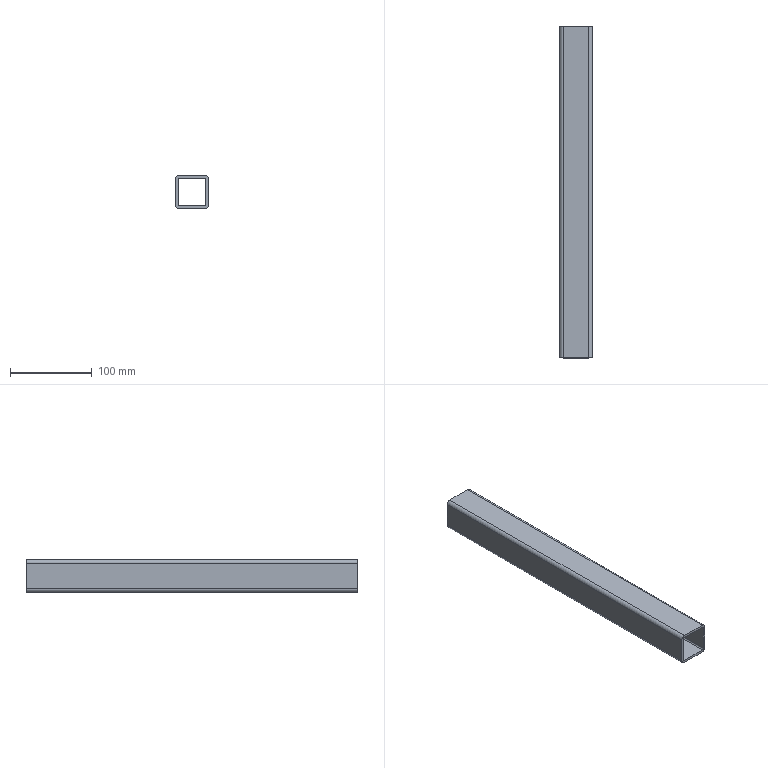Part | 1 solid | 18 faces | box 40 x 405 x 40 mm | volume 173562 mm3 | plane 10 | cylinder 8 | commonest cylinder face diameters 3 x4 9 x4
STEP:
#1=CARTESIAN_POINT('',(20.,0.,15.5));
#2=VERTEX_POINT('',#1);
#3=CARTESIAN_POINT('',(20.,0.,-15.5));
#4=VERTEX_POINT('',#3);
#5=CARTESIAN_POINT('',(20.,0.,20.));
#6=DIRECTION('',(0.,0.,-1.));
#7=VECTOR('',#6,1000.);
#8=LINE('',#5,#7);
#9=EDGE_CURVE('',#2,#4,#8,.T.);
#10=ORIENTED_EDGE('',*,*,#9,.T.);
#11=CARTESIAN_POINT('',(20.,405.,-15.5));
#12=VERTEX_POINT('',#11);
#13=CARTESIAN_POINT('',(20.,405.,-15.5));
#14=DIRECTION('',(0.,1.,0.));
#15=VECTOR('',#14,1000.);
#16=LINE('',#13,#15);
#17=EDGE_CURVE('',#4,#12,#16,.T.);
#18=ORIENTED_EDGE('',*,*,#17,.T.);
#19=CARTESIAN_POINT('',(20.,405.,15.5));
#20=VERTEX_POINT('',#19);
#21=CARTESIAN_POINT('',(20.,405.,20.));
#22=DIRECTION('',(0.,0.,-1.));
#23=VECTOR('',#22,1000.);
#24=LINE('',#21,#23);
#25=EDGE_CURVE('',#20,#12,#24,.T.);
#26=ORIENTED_EDGE('',*,*,#25,.F.);
#27=CARTESIAN_POINT('',(20.,405.,15.5));
#28=DIRECTION('',(0.,-1.,0.));
#29=VECTOR('',#28,1000.);
#30=LINE('',#27,#29);
#31=EDGE_CURVE('',#20,#2,#30,.T.);
#32=ORIENTED_EDGE('',*,*,#31,.T.);
#33=EDGE_LOOP('',(#10,#18,#26,#32));
#34=FACE_OUTER_BOUND('',#33,.T.);
#35=CARTESIAN_POINT('',(20.,405.,20.));
#36=DIRECTION('',(-1.,0.,0.));
#37=DIRECTION('',(0.,0.,1.));
#38=AXIS2_PLACEMENT_3D('',#35,#36,#37);
#39=PLANE('',#38);
#40=ADVANCED_FACE('',(#34),#39,.F.);
#41=CARTESIAN_POINT('',(15.5,0.,-20.));
#42=VERTEX_POINT('',#41);
#43=CARTESIAN_POINT('',(-15.5,0.,-20.));
#44=VERTEX_POINT('',#43);
#45=CARTESIAN_POINT('',(-20.,0.,-20.));
#46=DIRECTION('',(-1.,0.,0.));
#47=VECTOR('',#46,1000.);
#48=LINE('',#45,#47);
#49=EDGE_CURVE('',#42,#44,#48,.T.);
#50=ORIENTED_EDGE('',*,*,#49,.T.);
#51=CARTESIAN_POINT('',(-15.5,405.,-20.));
#52=VERTEX_POINT('',#51);
#53=CARTESIAN_POINT('',(-15.5,405.,-20.));
#54=DIRECTION('',(0.,1.,0.));
#55=VECTOR('',#54,1000.);
#56=LINE('',#53,#55);
#57=EDGE_CURVE('',#44,#52,#56,.T.);
#58=ORIENTED_EDGE('',*,*,#57,.T.);
#59=CARTESIAN_POINT('',(15.5,405.,-20.));
#60=VERTEX_POINT('',#59);
#61=CARTESIAN_POINT('',(-20.,405.,-20.));
#62=DIRECTION('',(-1.,0.,0.));
#63=VECTOR('',#62,1000.);
#64=LINE('',#61,#63);
#65=EDGE_CURVE('',#60,#52,#64,.T.);
#66=ORIENTED_EDGE('',*,*,#65,.F.);
#67=CARTESIAN_POINT('',(15.5,405.,-20.));
#68=DIRECTION('',(0.,-1.,0.));
#69=VECTOR('',#68,1000.);
#70=LINE('',#67,#69);
#71=EDGE_CURVE('',#60,#42,#70,.T.);
#72=ORIENTED_EDGE('',*,*,#71,.T.);
#73=EDGE_LOOP('',(#50,#58,#66,#72));
#74=FACE_OUTER_BOUND('',#73,.T.);
#75=CARTESIAN_POINT('',(-20.,405.,-20.));
#76=DIRECTION('',(0.,0.,1.));
#77=DIRECTION('',(1.,0.,0.));
#78=AXIS2_PLACEMENT_3D('',#75,#76,#77);
#79=PLANE('',#78);
#80=ADVANCED_FACE('',(#74),#79,.F.);
#81=CARTESIAN_POINT('',(-20.,0.,-15.5));
#82=VERTEX_POINT('',#81);
#83=CARTESIAN_POINT('',(-20.,0.,15.5));
#84=VERTEX_POINT('',#83);
#85=CARTESIAN_POINT('',(-20.,0.,20.));
#86=DIRECTION('',(0.,0.,1.));
#87=VECTOR('',#86,1000.);
#88=LINE('',#85,#87);
#89=EDGE_CURVE('',#82,#84,#88,.T.);
#90=ORIENTED_EDGE('',*,*,#89,.T.);
#91=CARTESIAN_POINT('',(-20.,405.,15.5));
#92=VERTEX_POINT('',#91);
#93=CARTESIAN_POINT('',(-20.,405.,15.5));
#94=DIRECTION('',(0.,1.,0.));
#95=VECTOR('',#94,1000.);
#96=LINE('',#93,#95);
#97=EDGE_CURVE('',#84,#92,#96,.T.);
#98=ORIENTED_EDGE('',*,*,#97,.T.);
#99=CARTESIAN_POINT('',(-20.,405.,-15.5));
#100=VERTEX_POINT('',#99);
#101=CARTESIAN_POINT('',(-20.,405.,20.));
#102=DIRECTION('',(0.,0.,1.));
#103=VECTOR('',#102,1000.);
#104=LINE('',#101,#103);
#105=EDGE_CURVE('',#100,#92,#104,.T.);
#106=ORIENTED_EDGE('',*,*,#105,.F.);
#107=CARTESIAN_POINT('',(-20.,405.,-15.5));
#108=DIRECTION('',(0.,-1.,0.));
#109=VECTOR('',#108,1000.);
#110=LINE('',#107,#109);
#111=EDGE_CURVE('',#100,#82,#110,.T.);
#112=ORIENTED_EDGE('',*,*,#111,.T.);
#113=EDGE_LOOP('',(#90,#98,#106,#112));
#114=FACE_OUTER_BOUND('',#113,.T.);
#115=CARTESIAN_POINT('',(-20.,405.,20.));
#116=DIRECTION('',(1.,0.,0.));
#117=DIRECTION('',(0.,0.,-1.));
#118=AXIS2_PLACEMENT_3D('',#115,#116,#117);
#119=PLANE('',#118);
#120=ADVANCED_FACE('',(#114),#119,.F.);
#121=CARTESIAN_POINT('',(-15.5,405.,20.));
#122=VERTEX_POINT('',#121);
#123=CARTESIAN_POINT('',(15.5,405.,20.));
#124=VERTEX_POINT('',#123);
#125=CARTESIAN_POINT('',(-20.,405.,20.));
#126=DIRECTION('',(1.,0.,0.));
#127=VECTOR('',#126,1000.);
#128=LINE('',#125,#127);
#129=EDGE_CURVE('',#122,#124,#128,.T.);
#130=ORIENTED_EDGE('',*,*,#129,.F.);
#131=CARTESIAN_POINT('',(-15.5,0.,20.));
#132=VERTEX_POINT('',#131);
#133=CARTESIAN_POINT('',(-15.5,405.,20.));
#134=DIRECTION('',(0.,-1.,0.));
#135=VECTOR('',#134,1000.);
#136=LINE('',#133,#135);
#137=EDGE_CURVE('',#122,#132,#136,.T.);
#138=ORIENTED_EDGE('',*,*,#137,.T.);
#139=CARTESIAN_POINT('',(15.5,0.,20.));
#140=VERTEX_POINT('',#139);
#141=CARTESIAN_POINT('',(-20.,0.,20.));
#142=DIRECTION('',(1.,0.,0.));
#143=VECTOR('',#142,1000.);
#144=LINE('',#141,#143);
#145=EDGE_CURVE('',#132,#140,#144,.T.);
#146=ORIENTED_EDGE('',*,*,#145,.T.);
#147=CARTESIAN_POINT('',(15.5,405.,20.));
#148=DIRECTION('',(0.,1.,0.));
#149=VECTOR('',#148,1000.);
#150=LINE('',#147,#149);
#151=EDGE_CURVE('',#140,#124,#150,.T.);
#152=ORIENTED_EDGE('',*,*,#151,.T.);
#153=EDGE_LOOP('',(#130,#138,#146,#152));
#154=FACE_OUTER_BOUND('',#153,.T.);
#155=CARTESIAN_POINT('',(-20.,405.,20.));
#156=DIRECTION('',(0.,0.,-1.));
#157=DIRECTION('',(-1.,0.,0.));
#158=AXIS2_PLACEMENT_3D('',#155,#156,#157);
#159=PLANE('',#158);
#160=ADVANCED_FACE('',(#154),#159,.F.);
#161=CARTESIAN_POINT('',(-17.,405.,-15.5));
#162=VERTEX_POINT('',#161);
#163=CARTESIAN_POINT('',(-17.,405.,15.5));
#164=VERTEX_POINT('',#163);
#165=CARTESIAN_POINT('',(-17.,405.,-15.5));
#166=DIRECTION('',(0.,0.,1.));
#167=VECTOR('',#166,1000.);
#168=LINE('',#165,#167);
#169=EDGE_CURVE('',#162,#164,#168,.T.);
#170=ORIENTED_EDGE('',*,*,#169,.F.);
#171=CARTESIAN_POINT('',(-15.5,405.,-17.));
#172=VERTEX_POINT('',#171);
#173=CARTESIAN_POINT('',(-15.5,405.,-15.5));
#174=DIRECTION('',(0.,1.,0.));
#175=DIRECTION('',(0.,0.,1.));
#176=AXIS2_PLACEMENT_3D('',#173,#174,#175);
#177=CIRCLE('',#176,1.5);
#178=EDGE_CURVE('',#172,#162,#177,.T.);
#179=ORIENTED_EDGE('',*,*,#178,.F.);
#180=CARTESIAN_POINT('',(15.5,405.,-17.));
#181=VERTEX_POINT('',#180);
#182=CARTESIAN_POINT('',(15.5,405.,-17.));
#183=DIRECTION('',(-1.,0.,0.));
#184=VECTOR('',#183,1000.);
#185=LINE('',#182,#184);
#186=EDGE_CURVE('',#181,#172,#185,.T.);
#187=ORIENTED_EDGE('',*,*,#186,.F.);
#188=CARTESIAN_POINT('',(17.,405.,-15.5));
#189=VERTEX_POINT('',#188);
#190=CARTESIAN_POINT('',(15.5,405.,-15.5));
#191=DIRECTION('',(0.,1.,0.));
#192=DIRECTION('',(0.,0.,1.));
#193=AXIS2_PLACEMENT_3D('',#190,#191,#192);
#194=CIRCLE('',#193,1.5);
#195=EDGE_CURVE('',#189,#181,#194,.T.);
#196=ORIENTED_EDGE('',*,*,#195,.F.);
#197=CARTESIAN_POINT('',(17.,405.,15.5));
#198=VERTEX_POINT('',#197);
#199=CARTESIAN_POINT('',(17.,405.,15.5));
#200=DIRECTION('',(0.,0.,-1.));
#201=VECTOR('',#200,1000.);
#202=LINE('',#199,#201);
#203=EDGE_CURVE('',#198,#189,#202,.T.);
#204=ORIENTED_EDGE('',*,*,#203,.F.);
#205=CARTESIAN_POINT('',(15.5,405.,17.));
#206=VERTEX_POINT('',#205);
#207=CARTESIAN_POINT('',(15.5,405.,15.5));
#208=DIRECTION('',(0.,1.,0.));
#209=DIRECTION('',(0.,0.,1.));
#210=AXIS2_PLACEMENT_3D('',#207,#208,#209);
#211=CIRCLE('',#210,1.5);
#212=EDGE_CURVE('',#206,#198,#211,.T.);
#213=ORIENTED_EDGE('',*,*,#212,.F.);
#214=CARTESIAN_POINT('',(-15.5,405.,17.));
#215=VERTEX_POINT('',#214);
#216=CARTESIAN_POINT('',(-15.5,405.,17.));
#217=DIRECTION('',(1.,0.,0.));
#218=VECTOR('',#217,1000.);
#219=LINE('',#216,#218);
#220=EDGE_CURVE('',#215,#206,#219,.T.);
#221=ORIENTED_EDGE('',*,*,#220,.F.);
#222=CARTESIAN_POINT('',(-15.5,405.,15.5));
#223=DIRECTION('',(0.,1.,0.));
#224=DIRECTION('',(0.,0.,1.));
#225=AXIS2_PLACEMENT_3D('',#222,#223,#224);
#226=CIRCLE('',#225,1.5);
#227=EDGE_CURVE('',#164,#215,#226,.T.);
#228=ORIENTED_EDGE('',*,*,#227,.F.);
#229=EDGE_LOOP('',(#170,#179,#187,#196,#204,#213,#221,#228));
#230=FACE_BOUND('',#229,.T.);
#231=ORIENTED_EDGE('',*,*,#105,.T.);
#232=CARTESIAN_POINT('',(-15.5,405.,15.5));
#233=DIRECTION('',(0.,1.,0.));
#234=DIRECTION('',(0.,0.,-1.));
#235=AXIS2_PLACEMENT_3D('',#232,#233,#234);
#236=CIRCLE('',#235,4.5);
#237=EDGE_CURVE('',#92,#122,#236,.T.);
#238=ORIENTED_EDGE('',*,*,#237,.T.);
#239=ORIENTED_EDGE('',*,*,#129,.T.);
#240=CARTESIAN_POINT('',(15.5,405.,15.5));
#241=DIRECTION('',(0.,1.,0.));
#242=DIRECTION('',(0.,0.,-1.));
#243=AXIS2_PLACEMENT_3D('',#240,#241,#242);
#244=CIRCLE('',#243,4.5);
#245=EDGE_CURVE('',#124,#20,#244,.T.);
#246=ORIENTED_EDGE('',*,*,#245,.T.);
#247=ORIENTED_EDGE('',*,*,#25,.T.);
#248=CARTESIAN_POINT('',(15.5,405.,-15.5));
#249=DIRECTION('',(0.,1.,0.));
#250=DIRECTION('',(0.,0.,-1.));
#251=AXIS2_PLACEMENT_3D('',#248,#249,#250);
#252=CIRCLE('',#251,4.5);
#253=EDGE_CURVE('',#12,#60,#252,.T.);
#254=ORIENTED_EDGE('',*,*,#253,.T.);
#255=ORIENTED_EDGE('',*,*,#65,.T.);
#256=CARTESIAN_POINT('',(-15.5,405.,-15.5));
#257=DIRECTION('',(0.,1.,0.));
#258=DIRECTION('',(0.,0.,-1.));
#259=AXIS2_PLACEMENT_3D('',#256,#257,#258);
#260=CIRCLE('',#259,4.5);
#261=EDGE_CURVE('',#52,#100,#260,.T.);
#262=ORIENTED_EDGE('',*,*,#261,.T.);
#263=EDGE_LOOP('',(#231,#238,#239,#246,#247,#254,#255,#262));
#264=FACE_OUTER_BOUND('',#263,.T.);
#265=CARTESIAN_POINT('',(0.,405.,0.));
#266=DIRECTION('',(0.,-1.,0.));
#267=DIRECTION('',(0.,0.,-1.));
#268=AXIS2_PLACEMENT_3D('',#265,#266,#267);
#269=PLANE('',#268);
#270=ADVANCED_FACE('',(#230,#264),#269,.F.);
#271=CARTESIAN_POINT('',(-15.5,0.,-17.));
#272=VERTEX_POINT('',#271);
#273=CARTESIAN_POINT('',(-17.,0.,-15.5));
#274=VERTEX_POINT('',#273);
#275=CARTESIAN_POINT('',(-15.5,0.,-15.5));
#276=DIRECTION('',(0.,1.,0.));
#277=DIRECTION('',(0.,0.,1.));
#278=AXIS2_PLACEMENT_3D('',#275,#276,#277);
#279=CIRCLE('',#278,1.5);
#280=EDGE_CURVE('',#272,#274,#279,.T.);
#281=ORIENTED_EDGE('',*,*,#280,.T.);
#282=CARTESIAN_POINT('',(-17.,0.,15.5));
#283=VERTEX_POINT('',#282);
#284=CARTESIAN_POINT('',(-17.,0.,-15.5));
#285=DIRECTION('',(0.,0.,1.));
#286=VECTOR('',#285,1000.);
#287=LINE('',#284,#286);
#288=EDGE_CURVE('',#274,#283,#287,.T.);
#289=ORIENTED_EDGE('',*,*,#288,.T.);
#290=CARTESIAN_POINT('',(-15.5,0.,17.));
#291=VERTEX_POINT('',#290);
#292=CARTESIAN_POINT('',(-15.5,0.,15.5));
#293=DIRECTION('',(0.,1.,0.));
#294=DIRECTION('',(0.,0.,1.));
#295=AXIS2_PLACEMENT_3D('',#292,#293,#294);
#296=CIRCLE('',#295,1.5);
#297=EDGE_CURVE('',#283,#291,#296,.T.);
#298=ORIENTED_EDGE('',*,*,#297,.T.);
#299=CARTESIAN_POINT('',(15.5,0.,17.));
#300=VERTEX_POINT('',#299);
#301=CARTESIAN_POINT('',(-15.5,0.,17.));
#302=DIRECTION('',(1.,0.,0.));
#303=VECTOR('',#302,1000.);
#304=LINE('',#301,#303);
#305=EDGE_CURVE('',#291,#300,#304,.T.);
#306=ORIENTED_EDGE('',*,*,#305,.T.);
#307=CARTESIAN_POINT('',(17.,0.,15.5));
#308=VERTEX_POINT('',#307);
#309=CARTESIAN_POINT('',(15.5,0.,15.5));
#310=DIRECTION('',(0.,1.,0.));
#311=DIRECTION('',(0.,0.,1.));
#312=AXIS2_PLACEMENT_3D('',#309,#310,#311);
#313=CIRCLE('',#312,1.5);
#314=EDGE_CURVE('',#300,#308,#313,.T.);
#315=ORIENTED_EDGE('',*,*,#314,.T.);
#316=CARTESIAN_POINT('',(17.,0.,-15.5));
#317=VERTEX_POINT('',#316);
#318=CARTESIAN_POINT('',(17.,0.,15.5));
#319=DIRECTION('',(0.,0.,-1.));
#320=VECTOR('',#319,1000.);
#321=LINE('',#318,#320);
#322=EDGE_CURVE('',#308,#317,#321,.T.);
#323=ORIENTED_EDGE('',*,*,#322,.T.);
#324=CARTESIAN_POINT('',(15.5,0.,-17.));
#325=VERTEX_POINT('',#324);
#326=CARTESIAN_POINT('',(15.5,0.,-15.5));
#327=DIRECTION('',(0.,1.,0.));
#328=DIRECTION('',(0.,0.,1.));
#329=AXIS2_PLACEMENT_3D('',#326,#327,#328);
#330=CIRCLE('',#329,1.5);
#331=EDGE_CURVE('',#317,#325,#330,.T.);
#332=ORIENTED_EDGE('',*,*,#331,.T.);
#333=CARTESIAN_POINT('',(15.5,0.,-17.));
#334=DIRECTION('',(-1.,0.,0.));
#335=VECTOR('',#334,1000.);
#336=LINE('',#333,#335);
#337=EDGE_CURVE('',#325,#272,#336,.T.);
#338=ORIENTED_EDGE('',*,*,#337,.T.);
#339=EDGE_LOOP('',(#281,#289,#298,#306,#315,#323,#332,#338));
#340=FACE_BOUND('',#339,.T.);
#341=ORIENTED_EDGE('',*,*,#145,.F.);
#342=CARTESIAN_POINT('',(-15.5,0.,15.5));
#343=DIRECTION('',(0.,-1.,0.));
#344=DIRECTION('',(0.,0.,-1.));
#345=AXIS2_PLACEMENT_3D('',#342,#343,#344);
#346=CIRCLE('',#345,4.5);
#347=EDGE_CURVE('',#132,#84,#346,.T.);
#348=ORIENTED_EDGE('',*,*,#347,.T.);
#349=ORIENTED_EDGE('',*,*,#89,.F.);
#350=CARTESIAN_POINT('',(-15.5,0.,-15.5));
#351=DIRECTION('',(0.,-1.,0.));
#352=DIRECTION('',(0.,0.,-1.));
#353=AXIS2_PLACEMENT_3D('',#350,#351,#352);
#354=CIRCLE('',#353,4.5);
#355=EDGE_CURVE('',#82,#44,#354,.T.);
#356=ORIENTED_EDGE('',*,*,#355,.T.);
#357=ORIENTED_EDGE('',*,*,#49,.F.);
#358=CARTESIAN_POINT('',(15.5,0.,-15.5));
#359=DIRECTION('',(0.,-1.,0.));
#360=DIRECTION('',(0.,0.,-1.));
#361=AXIS2_PLACEMENT_3D('',#358,#359,#360);
#362=CIRCLE('',#361,4.5);
#363=EDGE_CURVE('',#42,#4,#362,.T.);
#364=ORIENTED_EDGE('',*,*,#363,.T.);
#365=ORIENTED_EDGE('',*,*,#9,.F.);
#366=CARTESIAN_POINT('',(15.5,0.,15.5));
#367=DIRECTION('',(0.,-1.,0.));
#368=DIRECTION('',(0.,0.,-1.));
#369=AXIS2_PLACEMENT_3D('',#366,#367,#368);
#370=CIRCLE('',#369,4.5);
#371=EDGE_CURVE('',#2,#140,#370,.T.);
#372=ORIENTED_EDGE('',*,*,#371,.T.);
#373=EDGE_LOOP('',(#341,#348,#349,#356,#357,#364,#365,#372));
#374=FACE_OUTER_BOUND('',#373,.T.);
#375=CARTESIAN_POINT('',(0.,0.,0.));
#376=DIRECTION('',(0.,-1.,0.));
#377=DIRECTION('',(0.,0.,-1.));
#378=AXIS2_PLACEMENT_3D('',#375,#376,#377);
#379=PLANE('',#378);
#380=ADVANCED_FACE('',(#340,#374),#379,.T.);
#381=ORIENTED_EDGE('',*,*,#237,.F.);
#382=ORIENTED_EDGE('',*,*,#97,.F.);
#383=ORIENTED_EDGE('',*,*,#347,.F.);
#384=ORIENTED_EDGE('',*,*,#137,.F.);
#385=EDGE_LOOP('',(#381,#382,#383,#384));
#386=FACE_OUTER_BOUND('',#385,.T.);
#387=CARTESIAN_POINT('',(-15.5,405.,15.5));
#388=DIRECTION('',(0.,-1.,0.));
#389=DIRECTION('',(0.,0.,-1.));
#390=AXIS2_PLACEMENT_3D('',#387,#388,#389);
#391=CYLINDRICAL_SURFACE('',#390,4.5);
#392=ADVANCED_FACE('',(#386),#391,.T.);
#393=ORIENTED_EDGE('',*,*,#261,.F.);
#394=ORIENTED_EDGE('',*,*,#57,.F.);
#395=ORIENTED_EDGE('',*,*,#355,.F.);
#396=ORIENTED_EDGE('',*,*,#111,.F.);
#397=EDGE_LOOP('',(#393,#394,#395,#396));
#398=FACE_OUTER_BOUND('',#397,.T.);
#399=CARTESIAN_POINT('',(-15.5,405.,-15.5));
#400=DIRECTION('',(0.,-1.,0.));
#401=DIRECTION('',(0.,0.,-1.));
#402=AXIS2_PLACEMENT_3D('',#399,#400,#401);
#403=CYLINDRICAL_SURFACE('',#402,4.5);
#404=ADVANCED_FACE('',(#398),#403,.T.);
#405=ORIENTED_EDGE('',*,*,#253,.F.);
#406=ORIENTED_EDGE('',*,*,#17,.F.);
#407=ORIENTED_EDGE('',*,*,#363,.F.);
#408=ORIENTED_EDGE('',*,*,#71,.F.);
#409=EDGE_LOOP('',(#405,#406,#407,#408));
#410=FACE_OUTER_BOUND('',#409,.T.);
#411=CARTESIAN_POINT('',(15.5,405.,-15.5));
#412=DIRECTION('',(0.,-1.,0.));
#413=DIRECTION('',(0.,0.,-1.));
#414=AXIS2_PLACEMENT_3D('',#411,#412,#413);
#415=CYLINDRICAL_SURFACE('',#414,4.5);
#416=ADVANCED_FACE('',(#410),#415,.T.);
#417=ORIENTED_EDGE('',*,*,#245,.F.);
#418=ORIENTED_EDGE('',*,*,#151,.F.);
#419=ORIENTED_EDGE('',*,*,#371,.F.);
#420=ORIENTED_EDGE('',*,*,#31,.F.);
#421=EDGE_LOOP('',(#417,#418,#419,#420));
#422=FACE_OUTER_BOUND('',#421,.T.);
#423=CARTESIAN_POINT('',(15.5,405.,15.5));
#424=DIRECTION('',(0.,-1.,0.));
#425=DIRECTION('',(0.,0.,-1.));
#426=AXIS2_PLACEMENT_3D('',#423,#424,#425);
#427=CYLINDRICAL_SURFACE('',#426,4.5);
#428=ADVANCED_FACE('',(#422),#427,.T.);
#429=ORIENTED_EDGE('',*,*,#178,.T.);
#430=CARTESIAN_POINT('',(-17.,0.,-15.5));
#431=DIRECTION('',(0.,1.,0.));
#432=VECTOR('',#431,1000.);
#433=LINE('',#430,#432);
#434=EDGE_CURVE('',#274,#162,#433,.T.);
#435=ORIENTED_EDGE('',*,*,#434,.F.);
#436=ORIENTED_EDGE('',*,*,#280,.F.);
#437=CARTESIAN_POINT('',(-15.5,0.,-17.));
#438=DIRECTION('',(0.,1.,0.));
#439=VECTOR('',#438,1000.);
#440=LINE('',#437,#439);
#441=EDGE_CURVE('',#272,#172,#440,.T.);
#442=ORIENTED_EDGE('',*,*,#441,.T.);
#443=EDGE_LOOP('',(#429,#435,#436,#442));
#444=FACE_OUTER_BOUND('',#443,.T.);
#445=CARTESIAN_POINT('',(-15.5,0.,-15.5));
#446=DIRECTION('',(0.,1.,0.));
#447=DIRECTION('',(0.,0.,1.));
#448=AXIS2_PLACEMENT_3D('',#445,#446,#447);
#449=CYLINDRICAL_SURFACE('',#448,1.5);
#450=ADVANCED_FACE('',(#444),#449,.F.);
#451=ORIENTED_EDGE('',*,*,#186,.T.);
#452=ORIENTED_EDGE('',*,*,#441,.F.);
#453=ORIENTED_EDGE('',*,*,#337,.F.);
#454=CARTESIAN_POINT('',(15.5,0.,-17.));
#455=DIRECTION('',(0.,1.,0.));
#456=VECTOR('',#455,1000.);
#457=LINE('',#454,#456);
#458=EDGE_CURVE('',#325,#181,#457,.T.);
#459=ORIENTED_EDGE('',*,*,#458,.T.);
#460=EDGE_LOOP('',(#451,#452,#453,#459));
#461=FACE_OUTER_BOUND('',#460,.T.);
#462=CARTESIAN_POINT('',(15.5,0.,-17.));
#463=DIRECTION('',(0.,0.,-1.));
#464=DIRECTION('',(-1.,0.,0.));
#465=AXIS2_PLACEMENT_3D('',#462,#463,#464);
#466=PLANE('',#465);
#467=ADVANCED_FACE('',(#461),#466,.F.);
#468=ORIENTED_EDGE('',*,*,#195,.T.);
#469=ORIENTED_EDGE('',*,*,#458,.F.);
#470=ORIENTED_EDGE('',*,*,#331,.F.);
#471=CARTESIAN_POINT('',(17.,0.,-15.5));
#472=DIRECTION('',(0.,1.,0.));
#473=VECTOR('',#472,1000.);
#474=LINE('',#471,#473);
#475=EDGE_CURVE('',#317,#189,#474,.T.);
#476=ORIENTED_EDGE('',*,*,#475,.T.);
#477=EDGE_LOOP('',(#468,#469,#470,#476));
#478=FACE_OUTER_BOUND('',#477,.T.);
#479=CARTESIAN_POINT('',(15.5,0.,-15.5));
#480=DIRECTION('',(0.,1.,0.));
#481=DIRECTION('',(0.,0.,1.));
#482=AXIS2_PLACEMENT_3D('',#479,#480,#481);
#483=CYLINDRICAL_SURFACE('',#482,1.5);
#484=ADVANCED_FACE('',(#478),#483,.F.);
#485=ORIENTED_EDGE('',*,*,#203,.T.);
#486=ORIENTED_EDGE('',*,*,#475,.F.);
#487=ORIENTED_EDGE('',*,*,#322,.F.);
#488=CARTESIAN_POINT('',(17.,0.,15.5));
#489=DIRECTION('',(0.,1.,0.));
#490=VECTOR('',#489,1000.);
#491=LINE('',#488,#490);
#492=EDGE_CURVE('',#308,#198,#491,.T.);
#493=ORIENTED_EDGE('',*,*,#492,.T.);
#494=EDGE_LOOP('',(#485,#486,#487,#493));
#495=FACE_OUTER_BOUND('',#494,.T.);
#496=CARTESIAN_POINT('',(17.,0.,15.5));
#497=DIRECTION('',(1.,0.,0.));
#498=DIRECTION('',(0.,0.,-1.));
#499=AXIS2_PLACEMENT_3D('',#496,#497,#498);
#500=PLANE('',#499);
#501=ADVANCED_FACE('',(#495),#500,.F.);
#502=ORIENTED_EDGE('',*,*,#212,.T.);
#503=ORIENTED_EDGE('',*,*,#492,.F.);
#504=ORIENTED_EDGE('',*,*,#314,.F.);
#505=CARTESIAN_POINT('',(15.5,0.,17.));
#506=DIRECTION('',(0.,1.,0.));
#507=VECTOR('',#506,1000.);
#508=LINE('',#505,#507);
#509=EDGE_CURVE('',#300,#206,#508,.T.);
#510=ORIENTED_EDGE('',*,*,#509,.T.);
#511=EDGE_LOOP('',(#502,#503,#504,#510));
#512=FACE_OUTER_BOUND('',#511,.T.);
#513=CARTESIAN_POINT('',(15.5,0.,15.5));
#514=DIRECTION('',(0.,1.,0.));
#515=DIRECTION('',(0.,0.,1.));
#516=AXIS2_PLACEMENT_3D('',#513,#514,#515);
#517=CYLINDRICAL_SURFACE('',#516,1.5);
#518=ADVANCED_FACE('',(#512),#517,.F.);
#519=ORIENTED_EDGE('',*,*,#220,.T.);
#520=ORIENTED_EDGE('',*,*,#509,.F.);
#521=ORIENTED_EDGE('',*,*,#305,.F.);
#522=CARTESIAN_POINT('',(-15.5,0.,17.));
#523=DIRECTION('',(0.,1.,0.));
#524=VECTOR('',#523,1000.);
#525=LINE('',#522,#524);
#526=EDGE_CURVE('',#291,#215,#525,.T.);
#527=ORIENTED_EDGE('',*,*,#526,.T.);
#528=EDGE_LOOP('',(#519,#520,#521,#527));
#529=FACE_OUTER_BOUND('',#528,.T.);
#530=CARTESIAN_POINT('',(-15.5,0.,17.));
#531=DIRECTION('',(0.,0.,1.));
#532=DIRECTION('',(1.,0.,0.));
#533=AXIS2_PLACEMENT_3D('',#530,#531,#532);
#534=PLANE('',#533);
#535=ADVANCED_FACE('',(#529),#534,.F.);
#536=ORIENTED_EDGE('',*,*,#227,.T.);
#537=ORIENTED_EDGE('',*,*,#526,.F.);
#538=ORIENTED_EDGE('',*,*,#297,.F.);
#539=CARTESIAN_POINT('',(-17.,0.,15.5));
#540=DIRECTION('',(0.,1.,0.));
#541=VECTOR('',#540,1000.);
#542=LINE('',#539,#541);
#543=EDGE_CURVE('',#283,#164,#542,.T.);
#544=ORIENTED_EDGE('',*,*,#543,.T.);
#545=EDGE_LOOP('',(#536,#537,#538,#544));
#546=FACE_OUTER_BOUND('',#545,.T.);
#547=CARTESIAN_POINT('',(-15.5,0.,15.5));
#548=DIRECTION('',(0.,1.,0.));
#549=DIRECTION('',(0.,0.,1.));
#550=AXIS2_PLACEMENT_3D('',#547,#548,#549);
#551=CYLINDRICAL_SURFACE('',#550,1.5);
#552=ADVANCED_FACE('',(#546),#551,.F.);
#553=ORIENTED_EDGE('',*,*,#169,.T.);
#554=ORIENTED_EDGE('',*,*,#543,.F.);
#555=ORIENTED_EDGE('',*,*,#288,.F.);
#556=ORIENTED_EDGE('',*,*,#434,.T.);
#557=EDGE_LOOP('',(#553,#554,#555,#556));
#558=FACE_OUTER_BOUND('',#557,.T.);
#559=CARTESIAN_POINT('',(-17.,0.,-15.5));
#560=DIRECTION('',(-1.,0.,0.));
#561=DIRECTION('',(0.,0.,1.));
#562=AXIS2_PLACEMENT_3D('',#559,#560,#561);
#563=PLANE('',#562);
#564=ADVANCED_FACE('',(#558),#563,.F.);
#565=CLOSED_SHELL('',(#40,#80,#120,#160,#270,#380,#392,#404,#416,#428,#450,#467,#484,#501,#518,#535,#552,#564));
#566=MANIFOLD_SOLID_BREP('',#565);
#567=CARTESIAN_POINT('',(0.,0.,0.));
#568=DIRECTION('',(0.,0.,1.));
#569=DIRECTION('',(1.,0.,0.));
#570=AXIS2_PLACEMENT_3D('',#567,#568,#569);
#571=(LENGTH_UNIT()NAMED_UNIT(*)SI_UNIT(.MILLI.,.METRE.));
#572=UNCERTAINTY_MEASURE_WITH_UNIT(LENGTH_MEASURE(0.00001),#571,'','');
#573=(NAMED_UNIT(*)PLANE_ANGLE_UNIT()SI_UNIT($,.RADIAN.));
#574=(NAMED_UNIT(*)SI_UNIT($,.STERADIAN.)SOLID_ANGLE_UNIT());
#575=(GEOMETRIC_REPRESENTATION_CONTEXT(3)GLOBAL_UNCERTAINTY_ASSIGNED_CONTEXT((#572))GLOBAL_UNIT_ASSIGNED_CONTEXT((#571,#573,#574))REPRESENTATION_CONTEXT('',''));
#576=ADVANCED_BREP_SHAPE_REPRESENTATION('',(#566,#570),#575);